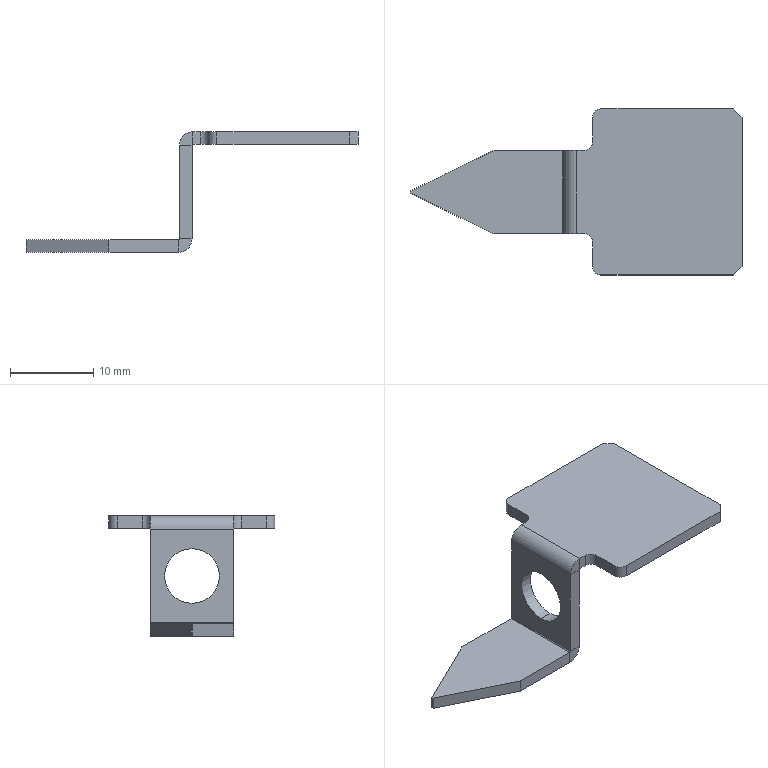Part | STEP file | Pointer | 1 solid | 36 faces | box 40 x 20 x 14.5 mm | volume 927.737 mm3 | plane 26 | cylinder 10 | commonest cylinder face diameters 2 x4 0.2 x2 3.2 x2 6.6 x2